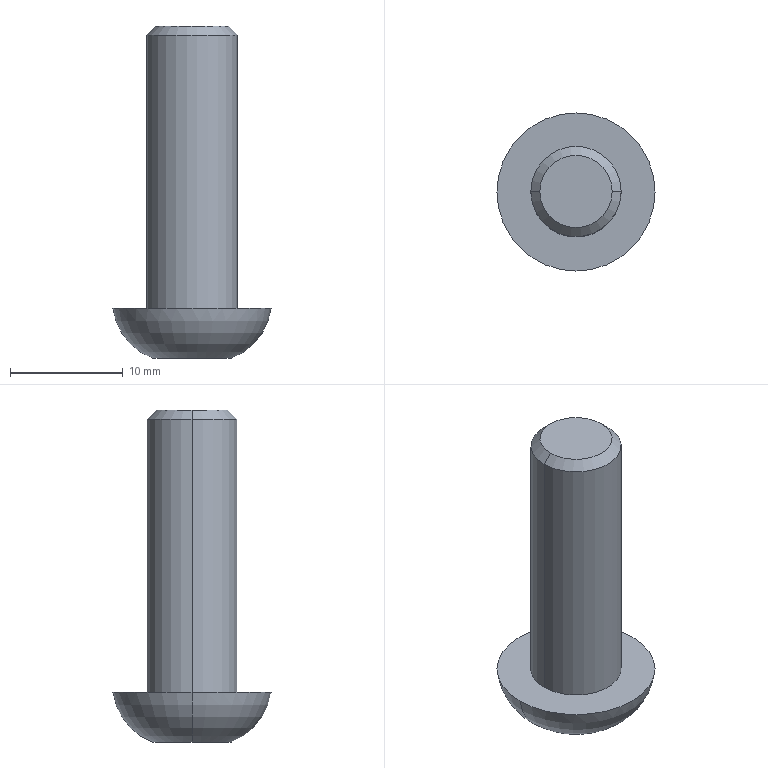Part | SolidWorks | features ICE 2, RevCut 2, Chamfer 1, Extrusion 1 | 1 solid | 23 faces | box 14 x 14 x 29.4 mm | volume 1691 mm3 | plane 15 | cone 4 | cylinder 2 | torus 2 | commonest cylinder face diameters 8 x2
STEP:
#1=CARTESIAN_POINT('',(-4.,0.,24.2));
#2=VERTEX_POINT('',#1);
#3=CARTESIAN_POINT('',(4.,0.,24.2));
#4=VERTEX_POINT('',#3);
#5=CARTESIAN_POINT('',(0.,0.,24.2));
#6=DIRECTION('',(0.,0.,-1.));
#7=DIRECTION('',(-1.,0.,0.));
#8=AXIS2_PLACEMENT_3D('',#5,#6,#7);
#9=CIRCLE('',#8,4.);
#10=EDGE_CURVE('',#2,#4,#9,.T.);
#11=ORIENTED_EDGE('',*,*,#10,.T.);
#12=CARTESIAN_POINT('',(4.,0.,0.));
#13=VERTEX_POINT('',#12);
#14=CARTESIAN_POINT('',(4.,0.,25.));
#15=DIRECTION('',(0.,0.,-1.));
#16=VECTOR('',#15,1000.);
#17=LINE('',#14,#16);
#18=EDGE_CURVE('',#4,#13,#17,.T.);
#19=ORIENTED_EDGE('',*,*,#18,.T.);
#20=CARTESIAN_POINT('',(-4.,0.,0.));
#21=VERTEX_POINT('',#20);
#22=CARTESIAN_POINT('',(0.,0.,0.));
#23=DIRECTION('',(0.,0.,1.));
#24=DIRECTION('',(1.,0.,0.));
#25=AXIS2_PLACEMENT_3D('',#22,#23,#24);
#26=CIRCLE('',#25,4.);
#27=EDGE_CURVE('',#13,#21,#26,.T.);
#28=ORIENTED_EDGE('',*,*,#27,.T.);
#29=CARTESIAN_POINT('',(-4.,0.,25.));
#30=DIRECTION('',(0.,0.,-1.));
#31=VECTOR('',#30,1000.);
#32=LINE('',#29,#31);
#33=EDGE_CURVE('',#2,#21,#32,.T.);
#34=ORIENTED_EDGE('',*,*,#33,.F.);
#35=EDGE_LOOP('',(#11,#19,#28,#34));
#36=FACE_OUTER_BOUND('',#35,.T.);
#37=CARTESIAN_POINT('',(0.,0.,25.));
#38=DIRECTION('',(0.,0.,-1.));
#39=DIRECTION('',(-1.,0.,0.));
#40=AXIS2_PLACEMENT_3D('',#37,#38,#39);
#41=CYLINDRICAL_SURFACE('',#40,4.);
#42=ADVANCED_FACE('',(#36),#41,.T.);
#43=CARTESIAN_POINT('',(3.2,0.,25.));
#44=VERTEX_POINT('',#43);
#45=CARTESIAN_POINT('',(-3.2,0.,25.));
#46=VERTEX_POINT('',#45);
#47=CARTESIAN_POINT('',(0.,0.,25.));
#48=DIRECTION('',(0.,0.,1.));
#49=DIRECTION('',(-1.,0.,0.));
#50=AXIS2_PLACEMENT_3D('',#47,#48,#49);
#51=CIRCLE('',#50,3.2);
#52=EDGE_CURVE('',#44,#46,#51,.T.);
#53=ORIENTED_EDGE('',*,*,#52,.F.);
#54=CARTESIAN_POINT('',(4.,0.,24.2));
#55=DIRECTION('',(0.7071,0.,-0.7071));
#56=VECTOR('',#55,1000.);
#57=LINE('',#54,#56);
#58=EDGE_CURVE('',#44,#4,#57,.T.);
#59=ORIENTED_EDGE('',*,*,#58,.T.);
#60=ORIENTED_EDGE('',*,*,#10,.F.);
#61=CARTESIAN_POINT('',(-4.,0.,24.2));
#62=DIRECTION('',(-0.7071,0.,-0.7071));
#63=VECTOR('',#62,1000.);
#64=LINE('',#61,#63);
#65=EDGE_CURVE('',#46,#2,#64,.T.);
#66=ORIENTED_EDGE('',*,*,#65,.F.);
#67=EDGE_LOOP('',(#53,#59,#60,#66));
#68=FACE_OUTER_BOUND('',#67,.T.);
#69=CARTESIAN_POINT('',(0.,0.,24.2));
#70=DIRECTION('',(0.,0.,-1.));
#71=DIRECTION('',(-1.,0.,0.));
#72=AXIS2_PLACEMENT_3D('',#69,#70,#71);
#73=CONICAL_SURFACE('',#72,4.,0.7854);
#74=ADVANCED_FACE('',(#68),#73,.T.);
#75=CARTESIAN_POINT('',(-7.,0.,0.));
#76=VERTEX_POINT('',#75);
#77=CARTESIAN_POINT('',(7.,0.,0.));
#78=VERTEX_POINT('',#77);
#79=CARTESIAN_POINT('',(0.,0.,0.));
#80=DIRECTION('',(0.,0.,-1.));
#81=DIRECTION('',(-1.,0.,0.));
#82=AXIS2_PLACEMENT_3D('',#79,#80,#81);
#83=CIRCLE('',#82,7.);
#84=EDGE_CURVE('',#76,#78,#83,.T.);
#85=ORIENTED_EDGE('',*,*,#84,.T.);
#86=CARTESIAN_POINT('',(3.5,0.,-4.4));
#87=VERTEX_POINT('',#86);
#88=CARTESIAN_POINT('',(1.642,0.,0.6702));
#89=DIRECTION('',(0.,1.,0.));
#90=DIRECTION('',(-1.,0.,0.));
#91=AXIS2_PLACEMENT_3D('',#88,#89,#90);
#92=CIRCLE('',#91,5.4);
#93=EDGE_CURVE('',#78,#87,#92,.T.);
#94=ORIENTED_EDGE('',*,*,#93,.T.);
#95=CARTESIAN_POINT('',(-3.5,0.,-4.4));
#96=VERTEX_POINT('',#95);
#97=CARTESIAN_POINT('',(0.,0.,-4.4));
#98=DIRECTION('',(0.,0.,-1.));
#99=DIRECTION('',(-1.,0.,0.));
#100=AXIS2_PLACEMENT_3D('',#97,#98,#99);
#101=CIRCLE('',#100,3.5);
#102=EDGE_CURVE('',#96,#87,#101,.T.);
#103=ORIENTED_EDGE('',*,*,#102,.F.);
#104=CARTESIAN_POINT('',(-1.642,0.,0.6702));
#105=DIRECTION('',(0.,-1.,0.));
#106=DIRECTION('',(0.,0.,-1.));
#107=AXIS2_PLACEMENT_3D('',#104,#105,#106);
#108=CIRCLE('',#107,5.4);
#109=EDGE_CURVE('',#76,#96,#108,.T.);
#110=ORIENTED_EDGE('',*,*,#109,.F.);
#111=EDGE_LOOP('',(#85,#94,#103,#110));
#112=FACE_OUTER_BOUND('',#111,.T.);
#113=CARTESIAN_POINT('',(0.,0.,0.6702));
#114=DIRECTION('',(0.,0.,-1.));
#115=DIRECTION('',(-1.,0.,0.));
#116=AXIS2_PLACEMENT_3D('',#113,#114,#115);
#117=TOROIDAL_SURFACE('',#116,1.642,5.4);
#118=ADVANCED_FACE('',(#112),#117,.T.);
#119=CARTESIAN_POINT('',(0.,0.,-0.7566));
#120=VERTEX_POINT('',#119);
#121=CARTESIAN_POINT('',(-2.5,0.,-2.2));
#122=VERTEX_POINT('',#121);
#123=CARTESIAN_POINT('',(-2.5,0.,-2.2));
#124=DIRECTION('',(-0.866,0.,-0.5));
#125=VECTOR('',#124,1000.);
#126=LINE('',#123,#125);
#127=EDGE_CURVE('',#120,#122,#126,.T.);
#128=ORIENTED_EDGE('',*,*,#127,.F.);
#129=CARTESIAN_POINT('',(2.5,0.,-2.2));
#130=VERTEX_POINT('',#129);
#131=CARTESIAN_POINT('',(2.5,0.,-2.2));
#132=DIRECTION('',(0.866,0.,-0.5));
#133=VECTOR('',#132,1000.);
#134=LINE('',#131,#133);
#135=EDGE_CURVE('',#120,#130,#134,.T.);
#136=ORIENTED_EDGE('',*,*,#135,.T.);
#137=CARTESIAN_POINT('',(2.165,-1.25,-2.2));
#138=VERTEX_POINT('',#137);
#139=CARTESIAN_POINT('',(0.,0.,-2.2));
#140=DIRECTION('',(0.,0.,1.));
#141=DIRECTION('',(1.,0.,0.));
#142=AXIS2_PLACEMENT_3D('',#139,#140,#141);
#143=CIRCLE('',#142,2.5);
#144=EDGE_CURVE('',#138,#130,#143,.T.);
#145=ORIENTED_EDGE('',*,*,#144,.F.);
#146=CARTESIAN_POINT('',(0.,-2.5,-2.2));
#147=VERTEX_POINT('',#146);
#148=CARTESIAN_POINT('',(0.,0.,-2.2));
#149=DIRECTION('',(0.,0.,1.));
#150=DIRECTION('',(1.,0.,0.));
#151=AXIS2_PLACEMENT_3D('',#148,#149,#150);
#152=CIRCLE('',#151,2.5);
#153=EDGE_CURVE('',#147,#138,#152,.T.);
#154=ORIENTED_EDGE('',*,*,#153,.F.);
#155=CARTESIAN_POINT('',(-2.165,-1.25,-2.2));
#156=VERTEX_POINT('',#155);
#157=CARTESIAN_POINT('',(0.,0.,-2.2));
#158=DIRECTION('',(0.,0.,1.));
#159=DIRECTION('',(1.,0.,0.));
#160=AXIS2_PLACEMENT_3D('',#157,#158,#159);
#161=CIRCLE('',#160,2.5);
#162=EDGE_CURVE('',#156,#147,#161,.T.);
#163=ORIENTED_EDGE('',*,*,#162,.F.);
#164=CARTESIAN_POINT('',(0.,0.,-2.2));
#165=DIRECTION('',(0.,0.,1.));
#166=DIRECTION('',(1.,0.,0.));
#167=AXIS2_PLACEMENT_3D('',#164,#165,#166);
#168=CIRCLE('',#167,2.5);
#169=EDGE_CURVE('',#122,#156,#168,.T.);
#170=ORIENTED_EDGE('',*,*,#169,.F.);
#171=EDGE_LOOP('',(#128,#136,#145,#154,#163,#170));
#172=FACE_OUTER_BOUND('',#171,.T.);
#173=CARTESIAN_POINT('',(0.,0.,-2.2));
#174=DIRECTION('',(0.,0.,-1.));
#175=DIRECTION('',(-1.,0.,0.));
#176=AXIS2_PLACEMENT_3D('',#173,#174,#175);
#177=CONICAL_SURFACE('',#176,2.5,1.047);
#178=ADVANCED_FACE('',(#172),#177,.F.);
#179=CARTESIAN_POINT('',(2.165,1.25,-2.2));
#180=VERTEX_POINT('',#179);
#181=CARTESIAN_POINT('',(1.443,2.5,-2.2));
#182=VERTEX_POINT('',#181);
#183=CARTESIAN_POINT('',(2.887,0.,-2.2));
#184=DIRECTION('',(-0.5,0.866,0.));
#185=VECTOR('',#184,1000.);
#186=LINE('',#183,#185);
#187=EDGE_CURVE('',#180,#182,#186,.T.);
#188=ORIENTED_EDGE('',*,*,#187,.F.);
#189=CARTESIAN_POINT('',(0.,2.5,-2.2));
#190=VERTEX_POINT('',#189);
#191=CARTESIAN_POINT('',(0.,0.,-2.2));
#192=DIRECTION('',(0.,0.,1.));
#193=DIRECTION('',(1.,0.,0.));
#194=AXIS2_PLACEMENT_3D('',#191,#192,#193);
#195=CIRCLE('',#194,2.5);
#196=EDGE_CURVE('',#180,#190,#195,.T.);
#197=ORIENTED_EDGE('',*,*,#196,.T.);
#198=CARTESIAN_POINT('',(1.443,2.5,-2.2));
#199=DIRECTION('',(-1.,0.,0.));
#200=VECTOR('',#199,1000.);
#201=LINE('',#198,#200);
#202=EDGE_CURVE('',#182,#190,#201,.T.);
#203=ORIENTED_EDGE('',*,*,#202,.F.);
#204=EDGE_LOOP('',(#188,#197,#203));
#205=FACE_OUTER_BOUND('',#204,.T.);
#206=CARTESIAN_POINT('',(0.,0.,-2.2));
#207=DIRECTION('',(0.,0.,1.));
#208=DIRECTION('',(1.,0.,0.));
#209=AXIS2_PLACEMENT_3D('',#206,#207,#208);
#210=PLANE('',#209);
#211=ADVANCED_FACE('',(#205),#210,.F.);
#212=CARTESIAN_POINT('',(-1.443,2.5,-2.2));
#213=VERTEX_POINT('',#212);
#214=CARTESIAN_POINT('',(1.443,2.5,-2.2));
#215=DIRECTION('',(-1.,0.,0.));
#216=VECTOR('',#215,1000.);
#217=LINE('',#214,#216);
#218=EDGE_CURVE('',#190,#213,#217,.T.);
#219=ORIENTED_EDGE('',*,*,#218,.F.);
#220=CARTESIAN_POINT('',(-2.165,1.25,-2.2));
#221=VERTEX_POINT('',#220);
#222=CARTESIAN_POINT('',(0.,0.,-2.2));
#223=DIRECTION('',(0.,0.,-1.));
#224=DIRECTION('',(-1.,0.,0.));
#225=AXIS2_PLACEMENT_3D('',#222,#223,#224);
#226=CIRCLE('',#225,2.5);
#227=EDGE_CURVE('',#221,#190,#226,.T.);
#228=ORIENTED_EDGE('',*,*,#227,.F.);
#229=CARTESIAN_POINT('',(-1.443,2.5,-2.2));
#230=DIRECTION('',(-0.5,-0.866,0.));
#231=VECTOR('',#230,1000.);
#232=LINE('',#229,#231);
#233=EDGE_CURVE('',#213,#221,#232,.T.);
#234=ORIENTED_EDGE('',*,*,#233,.F.);
#235=EDGE_LOOP('',(#219,#228,#234));
#236=FACE_OUTER_BOUND('',#235,.T.);
#237=CARTESIAN_POINT('',(0.,0.,-2.2));
#238=DIRECTION('',(0.,0.,1.));
#239=DIRECTION('',(1.,0.,0.));
#240=AXIS2_PLACEMENT_3D('',#237,#238,#239);
#241=PLANE('',#240);
#242=ADVANCED_FACE('',(#236),#241,.F.);
#243=CARTESIAN_POINT('',(-2.887,0.,-2.2));
#244=VERTEX_POINT('',#243);
#245=CARTESIAN_POINT('',(-1.443,2.5,-2.2));
#246=DIRECTION('',(-0.5,-0.866,0.));
#247=VECTOR('',#246,1000.);
#248=LINE('',#245,#247);
#249=EDGE_CURVE('',#221,#244,#248,.T.);
#250=ORIENTED_EDGE('',*,*,#249,.F.);
#251=CARTESIAN_POINT('',(0.,0.,-2.2));
#252=DIRECTION('',(0.,0.,1.));
#253=DIRECTION('',(1.,0.,0.));
#254=AXIS2_PLACEMENT_3D('',#251,#252,#253);
#255=CIRCLE('',#254,2.5);
#256=EDGE_CURVE('',#221,#122,#255,.T.);
#257=ORIENTED_EDGE('',*,*,#256,.T.);
#258=ORIENTED_EDGE('',*,*,#169,.T.);
#259=CARTESIAN_POINT('',(-2.887,0.,-2.2));
#260=DIRECTION('',(0.5,-0.866,0.));
#261=VECTOR('',#260,1000.);
#262=LINE('',#259,#261);
#263=EDGE_CURVE('',#244,#156,#262,.T.);
#264=ORIENTED_EDGE('',*,*,#263,.F.);
#265=EDGE_LOOP('',(#250,#257,#258,#264));
#266=FACE_OUTER_BOUND('',#265,.T.);
#267=CARTESIAN_POINT('',(0.,0.,-2.2));
#268=DIRECTION('',(0.,0.,1.));
#269=DIRECTION('',(1.,0.,0.));
#270=AXIS2_PLACEMENT_3D('',#267,#268,#269);
#271=PLANE('',#270);
#272=ADVANCED_FACE('',(#266),#271,.F.);
#273=CARTESIAN_POINT('',(-1.443,-2.5,-2.2));
#274=VERTEX_POINT('',#273);
#275=CARTESIAN_POINT('',(-2.887,0.,-2.2));
#276=DIRECTION('',(0.5,-0.866,0.));
#277=VECTOR('',#276,1000.);
#278=LINE('',#275,#277);
#279=EDGE_CURVE('',#156,#274,#278,.T.);
#280=ORIENTED_EDGE('',*,*,#279,.F.);
#281=ORIENTED_EDGE('',*,*,#162,.T.);
#282=CARTESIAN_POINT('',(-1.443,-2.5,-2.2));
#283=DIRECTION('',(1.,0.,0.));
#284=VECTOR('',#283,1000.);
#285=LINE('',#282,#284);
#286=EDGE_CURVE('',#274,#147,#285,.T.);
#287=ORIENTED_EDGE('',*,*,#286,.F.);
#288=EDGE_LOOP('',(#280,#281,#287));
#289=FACE_OUTER_BOUND('',#288,.T.);
#290=CARTESIAN_POINT('',(0.,0.,-2.2));
#291=DIRECTION('',(0.,0.,1.));
#292=DIRECTION('',(1.,0.,0.));
#293=AXIS2_PLACEMENT_3D('',#290,#291,#292);
#294=PLANE('',#293);
#295=ADVANCED_FACE('',(#289),#294,.F.);
#296=CARTESIAN_POINT('',(1.443,-2.5,-2.2));
#297=VERTEX_POINT('',#296);
#298=CARTESIAN_POINT('',(-1.443,-2.5,-2.2));
#299=DIRECTION('',(1.,0.,0.));
#300=VECTOR('',#299,1000.);
#301=LINE('',#298,#300);
#302=EDGE_CURVE('',#147,#297,#301,.T.);
#303=ORIENTED_EDGE('',*,*,#302,.F.);
#304=ORIENTED_EDGE('',*,*,#153,.T.);
#305=CARTESIAN_POINT('',(1.443,-2.5,-2.2));
#306=DIRECTION('',(0.5,0.866,0.));
#307=VECTOR('',#306,1000.);
#308=LINE('',#305,#307);
#309=EDGE_CURVE('',#297,#138,#308,.T.);
#310=ORIENTED_EDGE('',*,*,#309,.F.);
#311=EDGE_LOOP('',(#303,#304,#310));
#312=FACE_OUTER_BOUND('',#311,.T.);
#313=CARTESIAN_POINT('',(0.,0.,-2.2));
#314=DIRECTION('',(0.,0.,1.));
#315=DIRECTION('',(1.,0.,0.));
#316=AXIS2_PLACEMENT_3D('',#313,#314,#315);
#317=PLANE('',#316);
#318=ADVANCED_FACE('',(#312),#317,.F.);
#319=ORIENTED_EDGE('',*,*,#102,.T.);
#320=CARTESIAN_POINT('',(0.,0.,-4.4));
#321=DIRECTION('',(0.,0.,-1.));
#322=DIRECTION('',(-1.,0.,0.));
#323=AXIS2_PLACEMENT_3D('',#320,#321,#322);
#324=CIRCLE('',#323,3.5);
#325=EDGE_CURVE('',#87,#96,#324,.T.);
#326=ORIENTED_EDGE('',*,*,#325,.T.);
#327=EDGE_LOOP('',(#319,#326));
#328=FACE_OUTER_BOUND('',#327,.T.);
#329=CARTESIAN_POINT('',(2.887,0.,-4.4));
#330=VERTEX_POINT('',#329);
#331=CARTESIAN_POINT('',(1.443,2.5,-4.4));
#332=VERTEX_POINT('',#331);
#333=CARTESIAN_POINT('',(2.887,0.,-4.4));
#334=DIRECTION('',(-0.5,0.866,0.));
#335=VECTOR('',#334,1000.);
#336=LINE('',#333,#335);
#337=EDGE_CURVE('',#330,#332,#336,.T.);
#338=ORIENTED_EDGE('',*,*,#337,.T.);
#339=CARTESIAN_POINT('',(-1.443,2.5,-4.4));
#340=VERTEX_POINT('',#339);
#341=CARTESIAN_POINT('',(1.443,2.5,-4.4));
#342=DIRECTION('',(-1.,0.,0.));
#343=VECTOR('',#342,1000.);
#344=LINE('',#341,#343);
#345=EDGE_CURVE('',#332,#340,#344,.T.);
#346=ORIENTED_EDGE('',*,*,#345,.T.);
#347=CARTESIAN_POINT('',(-2.887,0.,-4.4));
#348=VERTEX_POINT('',#347);
#349=CARTESIAN_POINT('',(-1.443,2.5,-4.4));
#350=DIRECTION('',(-0.5,-0.866,0.));
#351=VECTOR('',#350,1000.);
#352=LINE('',#349,#351);
#353=EDGE_CURVE('',#340,#348,#352,.T.);
#354=ORIENTED_EDGE('',*,*,#353,.T.);
#355=CARTESIAN_POINT('',(-1.443,-2.5,-4.4));
#356=VERTEX_POINT('',#355);
#357=CARTESIAN_POINT('',(-2.887,0.,-4.4));
#358=DIRECTION('',(0.5,-0.866,0.));
#359=VECTOR('',#358,1000.);
#360=LINE('',#357,#359);
#361=EDGE_CURVE('',#348,#356,#360,.T.);
#362=ORIENTED_EDGE('',*,*,#361,.T.);
#363=CARTESIAN_POINT('',(1.443,-2.5,-4.4));
#364=VERTEX_POINT('',#363);
#365=CARTESIAN_POINT('',(-1.443,-2.5,-4.4));
#366=DIRECTION('',(1.,0.,0.));
#367=VECTOR('',#366,1000.);
#368=LINE('',#365,#367);
#369=EDGE_CURVE('',#356,#364,#368,.T.);
#370=ORIENTED_EDGE('',*,*,#369,.T.);
#371=CARTESIAN_POINT('',(1.443,-2.5,-4.4));
#372=DIRECTION('',(0.5,0.866,0.));
#373=VECTOR('',#372,1000.);
#374=LINE('',#371,#373);
#375=EDGE_CURVE('',#364,#330,#374,.T.);
#376=ORIENTED_EDGE('',*,*,#375,.T.);
#377=EDGE_LOOP('',(#338,#346,#354,#362,#370,#376));
#378=FACE_BOUND('',#377,.T.);
#379=CARTESIAN_POINT('',(0.,0.,-4.4));
#380=DIRECTION('',(0.,0.,1.));
#381=DIRECTION('',(1.,0.,0.));
#382=AXIS2_PLACEMENT_3D('',#379,#380,#381);
#383=PLANE('',#382);
#384=ADVANCED_FACE('',(#328,#378),#383,.F.);
#385=ORIENTED_EDGE('',*,*,#337,.F.);
#386=CARTESIAN_POINT('',(2.887,0.,-2.2));
#387=VERTEX_POINT('',#386);
#388=CARTESIAN_POINT('',(2.887,0.,-2.2));
#389=DIRECTION('',(0.,0.,-1.));
#390=VECTOR('',#389,1000.);
#391=LINE('',#388,#390);
#392=EDGE_CURVE('',#387,#330,#391,.T.);
#393=ORIENTED_EDGE('',*,*,#392,.F.);
#394=CARTESIAN_POINT('',(2.887,0.,-2.2));
#395=DIRECTION('',(-0.5,0.866,0.));
#396=VECTOR('',#395,1000.);
#397=LINE('',#394,#396);
#398=EDGE_CURVE('',#387,#180,#397,.T.);
#399=ORIENTED_EDGE('',*,*,#398,.T.);
#400=ORIENTED_EDGE('',*,*,#187,.T.);
#401=CARTESIAN_POINT('',(1.443,2.5,-2.2));
#402=DIRECTION('',(0.,0.,-1.));
#403=VECTOR('',#402,1000.);
#404=LINE('',#401,#403);
#405=EDGE_CURVE('',#182,#332,#404,.T.);
#406=ORIENTED_EDGE('',*,*,#405,.T.);
#407=EDGE_LOOP('',(#385,#393,#399,#400,#406));
#408=FACE_OUTER_BOUND('',#407,.T.);
#409=CARTESIAN_POINT('',(2.887,0.,-2.2));
#410=DIRECTION('',(-0.866,-0.5,0.));
#411=DIRECTION('',(0.5,-0.866,0.));
#412=AXIS2_PLACEMENT_3D('',#409,#410,#411);
#413=PLANE('',#412);
#414=ADVANCED_FACE('',(#408),#413,.T.);
#415=ORIENTED_EDGE('',*,*,#345,.F.);
#416=ORIENTED_EDGE('',*,*,#405,.F.);
#417=ORIENTED_EDGE('',*,*,#202,.T.);
#418=ORIENTED_EDGE('',*,*,#218,.T.);
#419=CARTESIAN_POINT('',(-1.443,2.5,-2.2));
#420=DIRECTION('',(0.,0.,-1.));
#421=VECTOR('',#420,1000.);
#422=LINE('',#419,#421);
#423=EDGE_CURVE('',#213,#340,#422,.T.);
#424=ORIENTED_EDGE('',*,*,#423,.T.);
#425=EDGE_LOOP('',(#415,#416,#417,#418,#424));
#426=FACE_OUTER_BOUND('',#425,.T.);
#427=CARTESIAN_POINT('',(1.443,2.5,-2.2));
#428=DIRECTION('',(0.,-1.,0.));
#429=DIRECTION('',(0.,0.,-1.));
#430=AXIS2_PLACEMENT_3D('',#427,#428,#429);
#431=PLANE('',#430);
#432=ADVANCED_FACE('',(#426),#431,.T.);
#433=ORIENTED_EDGE('',*,*,#353,.F.);
#434=ORIENTED_EDGE('',*,*,#423,.F.);
#435=ORIENTED_EDGE('',*,*,#233,.T.);
#436=ORIENTED_EDGE('',*,*,#249,.T.);
#437=CARTESIAN_POINT('',(-2.887,0.,-2.2));
#438=DIRECTION('',(0.,0.,-1.));
#439=VECTOR('',#438,1000.);
#440=LINE('',#437,#439);
#441=EDGE_CURVE('',#244,#348,#440,.T.);
#442=ORIENTED_EDGE('',*,*,#441,.T.);
#443=EDGE_LOOP('',(#433,#434,#435,#436,#442));
#444=FACE_OUTER_BOUND('',#443,.T.);
#445=CARTESIAN_POINT('',(-1.443,2.5,-2.2));
#446=DIRECTION('',(0.866,-0.5,0.));
#447=DIRECTION('',(0.5,0.866,0.));
#448=AXIS2_PLACEMENT_3D('',#445,#446,#447);
#449=PLANE('',#448);
#450=ADVANCED_FACE('',(#444),#449,.T.);
#451=ORIENTED_EDGE('',*,*,#361,.F.);
#452=ORIENTED_EDGE('',*,*,#441,.F.);
#453=ORIENTED_EDGE('',*,*,#263,.T.);
#454=ORIENTED_EDGE('',*,*,#279,.T.);
#455=CARTESIAN_POINT('',(-1.443,-2.5,-2.2));
#456=DIRECTION('',(0.,0.,-1.));
#457=VECTOR('',#456,1000.);
#458=LINE('',#455,#457);
#459=EDGE_CURVE('',#274,#356,#458,.T.);
#460=ORIENTED_EDGE('',*,*,#459,.T.);
#461=EDGE_LOOP('',(#451,#452,#453,#454,#460));
#462=FACE_OUTER_BOUND('',#461,.T.);
#463=CARTESIAN_POINT('',(-2.887,0.,-2.2));
#464=DIRECTION('',(0.866,0.5,0.));
#465=DIRECTION('',(-0.5,0.866,0.));
#466=AXIS2_PLACEMENT_3D('',#463,#464,#465);
#467=PLANE('',#466);
#468=ADVANCED_FACE('',(#462),#467,.T.);
#469=ORIENTED_EDGE('',*,*,#369,.F.);
#470=ORIENTED_EDGE('',*,*,#459,.F.);
#471=ORIENTED_EDGE('',*,*,#286,.T.);
#472=ORIENTED_EDGE('',*,*,#302,.T.);
#473=CARTESIAN_POINT('',(1.443,-2.5,-2.2));
#474=DIRECTION('',(0.,0.,-1.));
#475=VECTOR('',#474,1000.);
#476=LINE('',#473,#475);
#477=EDGE_CURVE('',#297,#364,#476,.T.);
#478=ORIENTED_EDGE('',*,*,#477,.T.);
#479=EDGE_LOOP('',(#469,#470,#471,#472,#478));
#480=FACE_OUTER_BOUND('',#479,.T.);
#481=CARTESIAN_POINT('',(-1.443,-2.5,-2.2));
#482=DIRECTION('',(0.,1.,0.));
#483=DIRECTION('',(0.,0.,1.));
#484=AXIS2_PLACEMENT_3D('',#481,#482,#483);
#485=PLANE('',#484);
#486=ADVANCED_FACE('',(#480),#485,.T.);
#487=ORIENTED_EDGE('',*,*,#375,.F.);
#488=ORIENTED_EDGE('',*,*,#477,.F.);
#489=ORIENTED_EDGE('',*,*,#309,.T.);
#490=CARTESIAN_POINT('',(1.443,-2.5,-2.2));
#491=DIRECTION('',(0.5,0.866,0.));
#492=VECTOR('',#491,1000.);
#493=LINE('',#490,#492);
#494=EDGE_CURVE('',#138,#387,#493,.T.);
#495=ORIENTED_EDGE('',*,*,#494,.T.);
#496=ORIENTED_EDGE('',*,*,#392,.T.);
#497=EDGE_LOOP('',(#487,#488,#489,#495,#496));
#498=FACE_OUTER_BOUND('',#497,.T.);
#499=CARTESIAN_POINT('',(1.443,-2.5,-2.2));
#500=DIRECTION('',(-0.866,0.5,0.));
#501=DIRECTION('',(-0.5,-0.866,0.));
#502=AXIS2_PLACEMENT_3D('',#499,#500,#501);
#503=PLANE('',#502);
#504=ADVANCED_FACE('',(#498),#503,.T.);
#505=ORIENTED_EDGE('',*,*,#494,.F.);
#506=ORIENTED_EDGE('',*,*,#144,.T.);
#507=CARTESIAN_POINT('',(0.,0.,-2.2));
#508=DIRECTION('',(0.,0.,1.));
#509=DIRECTION('',(1.,0.,0.));
#510=AXIS2_PLACEMENT_3D('',#507,#508,#509);
#511=CIRCLE('',#510,2.5);
#512=EDGE_CURVE('',#130,#180,#511,.T.);
#513=ORIENTED_EDGE('',*,*,#512,.T.);
#514=ORIENTED_EDGE('',*,*,#398,.F.);
#515=EDGE_LOOP('',(#505,#506,#513,#514));
#516=FACE_OUTER_BOUND('',#515,.T.);
#517=CARTESIAN_POINT('',(0.,0.,-2.2));
#518=DIRECTION('',(0.,0.,1.));
#519=DIRECTION('',(1.,0.,0.));
#520=AXIS2_PLACEMENT_3D('',#517,#518,#519);
#521=PLANE('',#520);
#522=ADVANCED_FACE('',(#516),#521,.F.);
#523=ORIENTED_EDGE('',*,*,#135,.F.);
#524=ORIENTED_EDGE('',*,*,#127,.T.);
#525=ORIENTED_EDGE('',*,*,#256,.F.);
#526=ORIENTED_EDGE('',*,*,#227,.T.);
#527=ORIENTED_EDGE('',*,*,#196,.F.);
#528=ORIENTED_EDGE('',*,*,#512,.F.);
#529=EDGE_LOOP('',(#523,#524,#525,#526,#527,#528));
#530=FACE_OUTER_BOUND('',#529,.T.);
#531=CARTESIAN_POINT('',(0.,0.,-2.2));
#532=DIRECTION('',(0.,0.,-1.));
#533=DIRECTION('',(-1.,0.,0.));
#534=AXIS2_PLACEMENT_3D('',#531,#532,#533);
#535=CONICAL_SURFACE('',#534,2.5,1.047);
#536=ADVANCED_FACE('',(#530),#535,.F.);
#537=ORIENTED_EDGE('',*,*,#93,.F.);
#538=CARTESIAN_POINT('',(0.,0.,0.));
#539=DIRECTION('',(0.,0.,-1.));
#540=DIRECTION('',(-1.,0.,0.));
#541=AXIS2_PLACEMENT_3D('',#538,#539,#540);
#542=CIRCLE('',#541,7.);
#543=EDGE_CURVE('',#78,#76,#542,.T.);
#544=ORIENTED_EDGE('',*,*,#543,.T.);
#545=ORIENTED_EDGE('',*,*,#109,.T.);
#546=ORIENTED_EDGE('',*,*,#325,.F.);
#547=EDGE_LOOP('',(#537,#544,#545,#546));
#548=FACE_OUTER_BOUND('',#547,.T.);
#549=CARTESIAN_POINT('',(0.,0.,0.6702));
#550=DIRECTION('',(0.,0.,-1.));
#551=DIRECTION('',(-1.,0.,0.));
#552=AXIS2_PLACEMENT_3D('',#549,#550,#551);
#553=TOROIDAL_SURFACE('',#552,1.642,5.4);
#554=ADVANCED_FACE('',(#548),#553,.T.);
#555=CARTESIAN_POINT('',(0.,0.,25.));
#556=DIRECTION('',(0.,0.,1.));
#557=DIRECTION('',(-1.,0.,0.));
#558=AXIS2_PLACEMENT_3D('',#555,#556,#557);
#559=CIRCLE('',#558,3.2);
#560=EDGE_CURVE('',#46,#44,#559,.T.);
#561=ORIENTED_EDGE('',*,*,#560,.T.);
#562=ORIENTED_EDGE('',*,*,#52,.T.);
#563=EDGE_LOOP('',(#561,#562));
#564=FACE_OUTER_BOUND('',#563,.T.);
#565=CARTESIAN_POINT('',(0.,0.,25.));
#566=DIRECTION('',(0.,0.,-1.));
#567=DIRECTION('',(-1.,0.,0.));
#568=AXIS2_PLACEMENT_3D('',#565,#566,#567);
#569=PLANE('',#568);
#570=ADVANCED_FACE('',(#564),#569,.F.);
#571=ORIENTED_EDGE('',*,*,#58,.F.);
#572=ORIENTED_EDGE('',*,*,#560,.F.);
#573=ORIENTED_EDGE('',*,*,#65,.T.);
#574=CARTESIAN_POINT('',(0.,0.,24.2));
#575=DIRECTION('',(0.,0.,-1.));
#576=DIRECTION('',(-1.,0.,0.));
#577=AXIS2_PLACEMENT_3D('',#574,#575,#576);
#578=CIRCLE('',#577,4.);
#579=EDGE_CURVE('',#4,#2,#578,.T.);
#580=ORIENTED_EDGE('',*,*,#579,.F.);
#581=EDGE_LOOP('',(#571,#572,#573,#580));
#582=FACE_OUTER_BOUND('',#581,.T.);
#583=CARTESIAN_POINT('',(0.,0.,24.2));
#584=DIRECTION('',(0.,0.,-1.));
#585=DIRECTION('',(-1.,0.,0.));
#586=AXIS2_PLACEMENT_3D('',#583,#584,#585);
#587=CONICAL_SURFACE('',#586,4.,0.7854);
#588=ADVANCED_FACE('',(#582),#587,.T.);
#589=ORIENTED_EDGE('',*,*,#18,.F.);
#590=ORIENTED_EDGE('',*,*,#579,.T.);
#591=ORIENTED_EDGE('',*,*,#33,.T.);
#592=CARTESIAN_POINT('',(0.,0.,0.));
#593=DIRECTION('',(0.,0.,1.));
#594=DIRECTION('',(1.,0.,0.));
#595=AXIS2_PLACEMENT_3D('',#592,#593,#594);
#596=CIRCLE('',#595,4.);
#597=EDGE_CURVE('',#21,#13,#596,.T.);
#598=ORIENTED_EDGE('',*,*,#597,.T.);
#599=EDGE_LOOP('',(#589,#590,#591,#598));
#600=FACE_OUTER_BOUND('',#599,.T.);
#601=CARTESIAN_POINT('',(0.,0.,25.));
#602=DIRECTION('',(0.,0.,-1.));
#603=DIRECTION('',(-1.,0.,0.));
#604=AXIS2_PLACEMENT_3D('',#601,#602,#603);
#605=CYLINDRICAL_SURFACE('',#604,4.);
#606=ADVANCED_FACE('',(#600),#605,.T.);
#607=ORIENTED_EDGE('',*,*,#597,.F.);
#608=ORIENTED_EDGE('',*,*,#27,.F.);
#609=EDGE_LOOP('',(#607,#608));
#610=FACE_BOUND('',#609,.T.);
#611=ORIENTED_EDGE('',*,*,#84,.F.);
#612=ORIENTED_EDGE('',*,*,#543,.F.);
#613=EDGE_LOOP('',(#611,#612));
#614=FACE_OUTER_BOUND('',#613,.T.);
#615=CARTESIAN_POINT('',(0.,0.,0.));
#616=DIRECTION('',(0.,0.,1.));
#617=DIRECTION('',(1.,0.,0.));
#618=AXIS2_PLACEMENT_3D('',#615,#616,#617);
#619=PLANE('',#618);
#620=ADVANCED_FACE('',(#610,#614),#619,.T.);
#621=CLOSED_SHELL('',(#42,#74,#118,#178,#211,#242,#272,#295,#318,#384,#414,#432,#450,#468,#486,#504,#522,#536,#554,#570,#588,#606,#620));
#622=MANIFOLD_SOLID_BREP('',#621);
#623=CARTESIAN_POINT('',(0.,0.,0.));
#624=DIRECTION('',(0.,0.,1.));
#625=DIRECTION('',(1.,0.,0.));
#626=AXIS2_PLACEMENT_3D('',#623,#624,#625);
#627=(LENGTH_UNIT()NAMED_UNIT(*)SI_UNIT(.MILLI.,.METRE.));
#628=UNCERTAINTY_MEASURE_WITH_UNIT(LENGTH_MEASURE(0.00001),#627,'','');
#629=(NAMED_UNIT(*)PLANE_ANGLE_UNIT()SI_UNIT($,.RADIAN.));
#630=(NAMED_UNIT(*)SI_UNIT($,.STERADIAN.)SOLID_ANGLE_UNIT());
#631=(GEOMETRIC_REPRESENTATION_CONTEXT(3)GLOBAL_UNCERTAINTY_ASSIGNED_CONTEXT((#628))GLOBAL_UNIT_ASSIGNED_CONTEXT((#627,#629,#630))REPRESENTATION_CONTEXT('',''));
#632=ADVANCED_BREP_SHAPE_REPRESENTATION('',(#622,#626),#631);